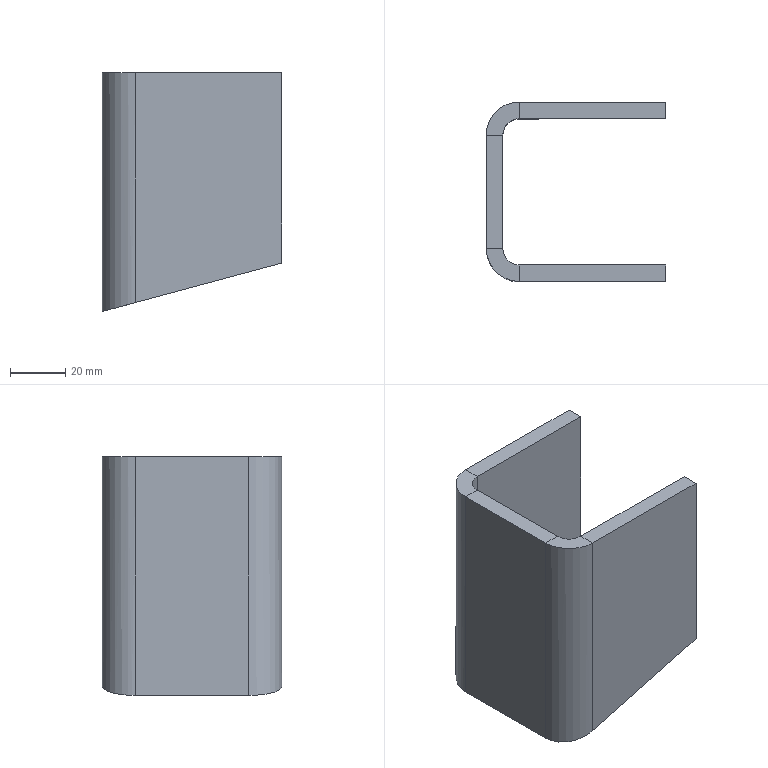Part | STEP file | 09-Bent plate | 1 solid | 18 faces | box 65 x 65 x 86.5 mm | volume 83900 mm3 | plane 14 | cylinder 4 | commonest cylinder face diameters 12 x2 24 x2
STEP:
#1=CARTESIAN_POINT('',(0.,0.,0.));
#2=DIRECTION('',(0.,0.,1.));
#3=DIRECTION('',(1.,0.,0.));
#4=AXIS2_PLACEMENT_3D('',#1,#2,#3);
#5=CARTESIAN_POINT('',(-53.,0.,86.5));
#6=VERTEX_POINT('',#5);
#7=CARTESIAN_POINT('',(-53.,-6.,86.5));
#8=VERTEX_POINT('',#7);
#9=CARTESIAN_POINT('',(-53.,0.,86.5));
#10=DIRECTION('',(0.,-1.,0.));
#11=VECTOR('',#10,1.);
#12=LINE('',#9,#11);
#13=CARTESIAN_POINT('',(-53.,0.,86.5));
#14=DIRECTION('',(0.,0.,1.));
#15=DIRECTION('',(1.,0.,0.));
#16=AXIS2_PLACEMENT_3D('',#13,#14,#15);
#17=PLANE('',#16);
#18=CARTESIAN_POINT('',(0.,0.));
#19=DIRECTION('',(0.,-1.));
#20=VECTOR('',#19,1.);
#21=LINE('',#18,#20);
#22=(GEOMETRIC_REPRESENTATION_CONTEXT(2)PARAMETRIC_REPRESENTATION_CONTEXT()REPRESENTATION_CONTEXT('',''));
#23=DEFINITIONAL_REPRESENTATION('',(#21),#22);
#24=PCURVE('',#17,#23);
#25=CARTESIAN_POINT('',(-59.,-12.,86.5));
#26=DIRECTION('',(0.,0.,1.));
#27=DIRECTION('',(1.,0.,0.));
#28=AXIS2_PLACEMENT_3D('',#25,#26,#27);
#29=PLANE('',#28);
#30=CARTESIAN_POINT('',(6.,12.));
#31=DIRECTION('',(0.,-1.));
#32=VECTOR('',#31,1.);
#33=LINE('',#30,#32);
#34=(GEOMETRIC_REPRESENTATION_CONTEXT(2)PARAMETRIC_REPRESENTATION_CONTEXT()REPRESENTATION_CONTEXT('',''));
#35=DEFINITIONAL_REPRESENTATION('',(#33),#34);
#36=PCURVE('',#29,#35);
#37=SURFACE_CURVE('',#12,(#24,#36),.PCURVE_S1.);
#38=EDGE_CURVE('',#6,#8,#37,.T.);
#39=ORIENTED_EDGE('',*,*,#38,.F.);
#40=CARTESIAN_POINT('',(-65.,-12.,86.5));
#41=VERTEX_POINT('',#40);
#42=CARTESIAN_POINT('',(-53.,-12.,86.5));
#43=DIRECTION('',(0.,0.,1.));
#44=DIRECTION('',(-1.,0.,0.));
#45=AXIS2_PLACEMENT_3D('',#42,#43,#44);
#46=CIRCLE('',#45,12.);
#47=CARTESIAN_POINT('',(0.,-12.));
#48=DIRECTION('',(-1.,0.));
#49=AXIS2_PLACEMENT_2D('',#47,#48);
#50=CIRCLE('',#49,12.);
#51=(GEOMETRIC_REPRESENTATION_CONTEXT(2)PARAMETRIC_REPRESENTATION_CONTEXT()REPRESENTATION_CONTEXT('',''));
#52=DEFINITIONAL_REPRESENTATION('',(#50),#51);
#53=PCURVE('',#17,#52);
#54=CARTESIAN_POINT('',(-53.,-12.,86.5));
#55=DIRECTION('',(0.,0.,-1.));
#56=DIRECTION('',(-1.,0.,0.));
#57=AXIS2_PLACEMENT_3D('',#54,#55,#56);
#58=CYLINDRICAL_SURFACE('',#57,12.);
#59=CARTESIAN_POINT('',(6.283,0.));
#60=DIRECTION('',(-1.,0.));
#61=VECTOR('',#60,1.);
#62=LINE('',#59,#61);
#63=(GEOMETRIC_REPRESENTATION_CONTEXT(2)PARAMETRIC_REPRESENTATION_CONTEXT()REPRESENTATION_CONTEXT('',''));
#64=DEFINITIONAL_REPRESENTATION('',(#62),#63);
#65=PCURVE('',#58,#64);
#66=SURFACE_CURVE('',#46,(#53,#65),.PCURVE_S1.);
#67=EDGE_CURVE('',#6,#41,#66,.T.);
#68=ORIENTED_EDGE('',*,*,#67,.T.);
#69=CARTESIAN_POINT('',(-59.,-12.,86.5));
#70=VERTEX_POINT('',#69);
#71=CARTESIAN_POINT('',(-59.,-12.,86.5));
#72=DIRECTION('',(-1.,0.,0.));
#73=VECTOR('',#72,1.);
#74=LINE('',#71,#73);
#75=CARTESIAN_POINT('',(-6.,-12.));
#76=DIRECTION('',(-1.,0.));
#77=VECTOR('',#76,1.);
#78=LINE('',#75,#77);
#79=(GEOMETRIC_REPRESENTATION_CONTEXT(2)PARAMETRIC_REPRESENTATION_CONTEXT()REPRESENTATION_CONTEXT('',''));
#80=DEFINITIONAL_REPRESENTATION('',(#78),#79);
#81=PCURVE('',#17,#80);
#82=CARTESIAN_POINT('',(-53.,-59.,86.5));
#83=DIRECTION('',(0.,0.,1.));
#84=DIRECTION('',(1.,0.,0.));
#85=AXIS2_PLACEMENT_3D('',#82,#83,#84);
#86=PLANE('',#85);
#87=CARTESIAN_POINT('',(-6.,47.));
#88=DIRECTION('',(-1.,0.));
#89=VECTOR('',#88,1.);
#90=LINE('',#87,#89);
#91=(GEOMETRIC_REPRESENTATION_CONTEXT(2)PARAMETRIC_REPRESENTATION_CONTEXT()REPRESENTATION_CONTEXT('',''));
#92=DEFINITIONAL_REPRESENTATION('',(#90),#91);
#93=PCURVE('',#86,#92);
#94=SURFACE_CURVE('',#74,(#81,#93),.PCURVE_S1.);
#95=EDGE_CURVE('',#70,#41,#94,.T.);
#96=ORIENTED_EDGE('',*,*,#95,.F.);
#97=CARTESIAN_POINT('',(-53.,-12.,86.5));
#98=DIRECTION('',(0.,0.,1.));
#99=DIRECTION('',(1.,0.,0.));
#100=AXIS2_PLACEMENT_3D('',#97,#98,#99);
#101=CIRCLE('',#100,6.);
#102=CARTESIAN_POINT('',(0.,-12.));
#103=DIRECTION('',(1.,0.));
#104=AXIS2_PLACEMENT_2D('',#102,#103);
#105=CIRCLE('',#104,6.);
#106=(GEOMETRIC_REPRESENTATION_CONTEXT(2)PARAMETRIC_REPRESENTATION_CONTEXT()REPRESENTATION_CONTEXT('',''));
#107=DEFINITIONAL_REPRESENTATION('',(#105),#106);
#108=PCURVE('',#17,#107);
#109=CARTESIAN_POINT('',(-53.,-12.,86.5));
#110=DIRECTION('',(0.,0.,-1.));
#111=DIRECTION('',(-1.,0.,0.));
#112=AXIS2_PLACEMENT_3D('',#109,#110,#111);
#113=CYLINDRICAL_SURFACE('',#112,6.);
#114=CARTESIAN_POINT('',(3.142,0.));
#115=DIRECTION('',(-1.,0.));
#116=VECTOR('',#115,1.);
#117=LINE('',#114,#116);
#118=(GEOMETRIC_REPRESENTATION_CONTEXT(2)PARAMETRIC_REPRESENTATION_CONTEXT()REPRESENTATION_CONTEXT('',''));
#119=DEFINITIONAL_REPRESENTATION('',(#117),#118);
#120=PCURVE('',#113,#119);
#121=SURFACE_CURVE('',#101,(#108,#120),.PCURVE_S1.);
#122=EDGE_CURVE('',#8,#70,#121,.T.);
#123=ORIENTED_EDGE('',*,*,#122,.F.);
#124=EDGE_LOOP('',(#39,#68,#96,#123));
#125=FACE_BOUND('',#124,.T.);
#126=ADVANCED_FACE('',(#125),#17,.T.);
#127=CARTESIAN_POINT('',(0.,0.,86.5));
#128=VERTEX_POINT('',#127);
#129=CARTESIAN_POINT('',(0.,0.,86.5));
#130=DIRECTION('',(-1.,0.,0.));
#131=VECTOR('',#130,1.);
#132=LINE('',#129,#131);
#133=CARTESIAN_POINT('',(59.,12.));
#134=DIRECTION('',(-1.,0.));
#135=VECTOR('',#134,1.);
#136=LINE('',#133,#135);
#137=(GEOMETRIC_REPRESENTATION_CONTEXT(2)PARAMETRIC_REPRESENTATION_CONTEXT()REPRESENTATION_CONTEXT('',''));
#138=DEFINITIONAL_REPRESENTATION('',(#136),#137);
#139=PCURVE('',#29,#138);
#140=CARTESIAN_POINT('',(0.,0.,86.5));
#141=DIRECTION('',(0.,-1.,0.));
#142=DIRECTION('',(1.,0.,0.));
#143=AXIS2_PLACEMENT_3D('',#140,#141,#142);
#144=PLANE('',#143);
#145=CARTESIAN_POINT('',(0.,0.));
#146=DIRECTION('',(-1.,0.));
#147=VECTOR('',#146,1.);
#148=LINE('',#145,#147);
#149=(GEOMETRIC_REPRESENTATION_CONTEXT(2)PARAMETRIC_REPRESENTATION_CONTEXT()REPRESENTATION_CONTEXT('',''));
#150=DEFINITIONAL_REPRESENTATION('',(#148),#149);
#151=PCURVE('',#144,#150);
#152=SURFACE_CURVE('',#132,(#139,#151),.PCURVE_S1.);
#153=EDGE_CURVE('',#128,#6,#152,.T.);
#154=ORIENTED_EDGE('',*,*,#153,.T.);
#155=ORIENTED_EDGE('',*,*,#38,.T.);
#156=CARTESIAN_POINT('',(0.,-6.,86.5));
#157=VERTEX_POINT('',#156);
#158=CARTESIAN_POINT('',(0.,-6.,86.5));
#159=DIRECTION('',(-1.,0.,0.));
#160=VECTOR('',#159,1.);
#161=LINE('',#158,#160);
#162=CARTESIAN_POINT('',(59.,6.));
#163=DIRECTION('',(-1.,0.));
#164=VECTOR('',#163,1.);
#165=LINE('',#162,#164);
#166=(GEOMETRIC_REPRESENTATION_CONTEXT(2)PARAMETRIC_REPRESENTATION_CONTEXT()REPRESENTATION_CONTEXT('',''));
#167=DEFINITIONAL_REPRESENTATION('',(#165),#166);
#168=PCURVE('',#29,#167);
#169=CARTESIAN_POINT('',(0.,-6.,86.5));
#170=DIRECTION('',(0.,-1.,0.));
#171=DIRECTION('',(1.,0.,0.));
#172=AXIS2_PLACEMENT_3D('',#169,#170,#171);
#173=PLANE('',#172);
#174=CARTESIAN_POINT('',(0.,0.));
#175=DIRECTION('',(-1.,0.));
#176=VECTOR('',#175,1.);
#177=LINE('',#174,#176);
#178=(GEOMETRIC_REPRESENTATION_CONTEXT(2)PARAMETRIC_REPRESENTATION_CONTEXT()REPRESENTATION_CONTEXT('',''));
#179=DEFINITIONAL_REPRESENTATION('',(#177),#178);
#180=PCURVE('',#173,#179);
#181=SURFACE_CURVE('',#161,(#168,#180),.PCURVE_S1.);
#182=EDGE_CURVE('',#157,#8,#181,.T.);
#183=ORIENTED_EDGE('',*,*,#182,.F.);
#184=CARTESIAN_POINT('',(0.,0.,86.5));
#185=DIRECTION('',(0.,-1.,0.));
#186=VECTOR('',#185,1.);
#187=LINE('',#184,#186);
#188=CARTESIAN_POINT('',(59.,12.));
#189=DIRECTION('',(0.,-1.));
#190=VECTOR('',#189,1.);
#191=LINE('',#188,#190);
#192=(GEOMETRIC_REPRESENTATION_CONTEXT(2)PARAMETRIC_REPRESENTATION_CONTEXT()REPRESENTATION_CONTEXT('',''));
#193=DEFINITIONAL_REPRESENTATION('',(#191),#192);
#194=PCURVE('',#29,#193);
#195=CARTESIAN_POINT('',(0.,0.,86.5));
#196=DIRECTION('',(1.,0.,0.));
#197=DIRECTION('',(0.,1.,0.));
#198=AXIS2_PLACEMENT_3D('',#195,#196,#197);
#199=PLANE('',#198);
#200=CARTESIAN_POINT('',(0.,0.));
#201=DIRECTION('',(-1.,0.));
#202=VECTOR('',#201,1.);
#203=LINE('',#200,#202);
#204=(GEOMETRIC_REPRESENTATION_CONTEXT(2)PARAMETRIC_REPRESENTATION_CONTEXT()REPRESENTATION_CONTEXT('',''));
#205=DEFINITIONAL_REPRESENTATION('',(#203),#204);
#206=PCURVE('',#199,#205);
#207=SURFACE_CURVE('',#187,(#194,#206),.PCURVE_S1.);
#208=EDGE_CURVE('',#128,#157,#207,.T.);
#209=ORIENTED_EDGE('',*,*,#208,.F.);
#210=EDGE_LOOP('',(#154,#155,#183,#209));
#211=FACE_BOUND('',#210,.T.);
#212=ADVANCED_FACE('',(#211),#29,.T.);
#213=CARTESIAN_POINT('',(-65.,-53.,86.5));
#214=VERTEX_POINT('',#213);
#215=CARTESIAN_POINT('',(-59.,-53.,86.5));
#216=VERTEX_POINT('',#215);
#217=CARTESIAN_POINT('',(-65.,-53.,86.5));
#218=DIRECTION('',(1.,0.,0.));
#219=VECTOR('',#218,1.);
#220=LINE('',#217,#219);
#221=CARTESIAN_POINT('',(-65.,-53.,86.5));
#222=DIRECTION('',(0.,0.,1.));
#223=DIRECTION('',(1.,0.,0.));
#224=AXIS2_PLACEMENT_3D('',#221,#222,#223);
#225=PLANE('',#224);
#226=CARTESIAN_POINT('',(0.,0.));
#227=DIRECTION('',(1.,0.));
#228=VECTOR('',#227,1.);
#229=LINE('',#226,#228);
#230=(GEOMETRIC_REPRESENTATION_CONTEXT(2)PARAMETRIC_REPRESENTATION_CONTEXT()REPRESENTATION_CONTEXT('',''));
#231=DEFINITIONAL_REPRESENTATION('',(#229),#230);
#232=PCURVE('',#225,#231);
#233=CARTESIAN_POINT('',(-12.,6.));
#234=DIRECTION('',(1.,0.));
#235=VECTOR('',#234,1.);
#236=LINE('',#233,#235);
#237=(GEOMETRIC_REPRESENTATION_CONTEXT(2)PARAMETRIC_REPRESENTATION_CONTEXT()REPRESENTATION_CONTEXT('',''));
#238=DEFINITIONAL_REPRESENTATION('',(#236),#237);
#239=PCURVE('',#86,#238);
#240=SURFACE_CURVE('',#220,(#232,#239),.PCURVE_S1.);
#241=EDGE_CURVE('',#214,#216,#240,.T.);
#242=ORIENTED_EDGE('',*,*,#241,.F.);
#243=CARTESIAN_POINT('',(-53.,-65.,86.5));
#244=VERTEX_POINT('',#243);
#245=CARTESIAN_POINT('',(-53.,-53.,86.5));
#246=DIRECTION('',(0.,0.,1.));
#247=DIRECTION('',(-1.,0.,0.));
#248=AXIS2_PLACEMENT_3D('',#245,#246,#247);
#249=CIRCLE('',#248,12.);
#250=CARTESIAN_POINT('',(12.,0.));
#251=DIRECTION('',(-1.,0.));
#252=AXIS2_PLACEMENT_2D('',#250,#251);
#253=CIRCLE('',#252,12.);
#254=(GEOMETRIC_REPRESENTATION_CONTEXT(2)PARAMETRIC_REPRESENTATION_CONTEXT()REPRESENTATION_CONTEXT('',''));
#255=DEFINITIONAL_REPRESENTATION('',(#253),#254);
#256=PCURVE('',#225,#255);
#257=CARTESIAN_POINT('',(-53.,-53.,86.5));
#258=DIRECTION('',(0.,0.,-1.));
#259=DIRECTION('',(-1.,0.,0.));
#260=AXIS2_PLACEMENT_3D('',#257,#258,#259);
#261=CYLINDRICAL_SURFACE('',#260,12.);
#262=CARTESIAN_POINT('',(6.283,0.));
#263=DIRECTION('',(-1.,0.));
#264=VECTOR('',#263,1.);
#265=LINE('',#262,#264);
#266=(GEOMETRIC_REPRESENTATION_CONTEXT(2)PARAMETRIC_REPRESENTATION_CONTEXT()REPRESENTATION_CONTEXT('',''));
#267=DEFINITIONAL_REPRESENTATION('',(#265),#266);
#268=PCURVE('',#261,#267);
#269=SURFACE_CURVE('',#249,(#256,#268),.PCURVE_S1.);
#270=EDGE_CURVE('',#214,#244,#269,.T.);
#271=ORIENTED_EDGE('',*,*,#270,.T.);
#272=CARTESIAN_POINT('',(-53.,-59.,86.5));
#273=VERTEX_POINT('',#272);
#274=CARTESIAN_POINT('',(-53.,-59.,86.5));
#275=DIRECTION('',(0.,-1.,0.));
#276=VECTOR('',#275,1.);
#277=LINE('',#274,#276);
#278=CARTESIAN_POINT('',(12.,-6.));
#279=DIRECTION('',(0.,-1.));
#280=VECTOR('',#279,1.);
#281=LINE('',#278,#280);
#282=(GEOMETRIC_REPRESENTATION_CONTEXT(2)PARAMETRIC_REPRESENTATION_CONTEXT()REPRESENTATION_CONTEXT('',''));
#283=DEFINITIONAL_REPRESENTATION('',(#281),#282);
#284=PCURVE('',#225,#283);
#285=CARTESIAN_POINT('',(-53.,-53.,86.5));
#286=DIRECTION('',(0.,0.,1.));
#287=DIRECTION('',(1.,0.,0.));
#288=AXIS2_PLACEMENT_3D('',#285,#286,#287);
#289=PLANE('',#288);
#290=CARTESIAN_POINT('',(0.,-6.));
#291=DIRECTION('',(0.,-1.));
#292=VECTOR('',#291,1.);
#293=LINE('',#290,#292);
#294=(GEOMETRIC_REPRESENTATION_CONTEXT(2)PARAMETRIC_REPRESENTATION_CONTEXT()REPRESENTATION_CONTEXT('',''));
#295=DEFINITIONAL_REPRESENTATION('',(#293),#294);
#296=PCURVE('',#289,#295);
#297=SURFACE_CURVE('',#277,(#284,#296),.PCURVE_S1.);
#298=EDGE_CURVE('',#273,#244,#297,.T.);
#299=ORIENTED_EDGE('',*,*,#298,.F.);
#300=CARTESIAN_POINT('',(-53.,-53.,86.5));
#301=DIRECTION('',(0.,0.,1.));
#302=DIRECTION('',(1.,0.,0.));
#303=AXIS2_PLACEMENT_3D('',#300,#301,#302);
#304=CIRCLE('',#303,6.);
#305=CARTESIAN_POINT('',(12.,0.));
#306=DIRECTION('',(1.,0.));
#307=AXIS2_PLACEMENT_2D('',#305,#306);
#308=CIRCLE('',#307,6.);
#309=(GEOMETRIC_REPRESENTATION_CONTEXT(2)PARAMETRIC_REPRESENTATION_CONTEXT()REPRESENTATION_CONTEXT('',''));
#310=DEFINITIONAL_REPRESENTATION('',(#308),#309);
#311=PCURVE('',#225,#310);
#312=CARTESIAN_POINT('',(-53.,-53.,86.5));
#313=DIRECTION('',(0.,0.,-1.));
#314=DIRECTION('',(-1.,0.,0.));
#315=AXIS2_PLACEMENT_3D('',#312,#313,#314);
#316=CYLINDRICAL_SURFACE('',#315,6.);
#317=CARTESIAN_POINT('',(9.425,0.));
#318=DIRECTION('',(-1.,0.));
#319=VECTOR('',#318,1.);
#320=LINE('',#317,#319);
#321=(GEOMETRIC_REPRESENTATION_CONTEXT(2)PARAMETRIC_REPRESENTATION_CONTEXT()REPRESENTATION_CONTEXT('',''));
#322=DEFINITIONAL_REPRESENTATION('',(#320),#321);
#323=PCURVE('',#316,#322);
#324=SURFACE_CURVE('',#304,(#311,#323),.PCURVE_S1.);
#325=EDGE_CURVE('',#216,#273,#324,.T.);
#326=ORIENTED_EDGE('',*,*,#325,.F.);
#327=EDGE_LOOP('',(#242,#271,#299,#326));
#328=FACE_BOUND('',#327,.T.);
#329=ADVANCED_FACE('',(#328),#225,.T.);
#330=CARTESIAN_POINT('',(-65.,0.,86.5));
#331=DIRECTION('',(0.,-1.,0.));
#332=VECTOR('',#331,1.);
#333=LINE('',#330,#332);
#334=CARTESIAN_POINT('',(-12.,59.));
#335=DIRECTION('',(0.,-1.));
#336=VECTOR('',#335,1.);
#337=LINE('',#334,#336);
#338=(GEOMETRIC_REPRESENTATION_CONTEXT(2)PARAMETRIC_REPRESENTATION_CONTEXT()REPRESENTATION_CONTEXT('',''));
#339=DEFINITIONAL_REPRESENTATION('',(#337),#338);
#340=PCURVE('',#86,#339);
#341=CARTESIAN_POINT('',(-65.,0.,86.5));
#342=DIRECTION('',(1.,0.,0.));
#343=DIRECTION('',(0.,1.,0.));
#344=AXIS2_PLACEMENT_3D('',#341,#342,#343);
#345=PLANE('',#344);
#346=CARTESIAN_POINT('',(0.,0.));
#347=DIRECTION('',(-1.,0.));
#348=VECTOR('',#347,1.);
#349=LINE('',#346,#348);
#350=(GEOMETRIC_REPRESENTATION_CONTEXT(2)PARAMETRIC_REPRESENTATION_CONTEXT()REPRESENTATION_CONTEXT('',''));
#351=DEFINITIONAL_REPRESENTATION('',(#349),#350);
#352=PCURVE('',#345,#351);
#353=SURFACE_CURVE('',#333,(#340,#352),.PCURVE_S1.);
#354=EDGE_CURVE('',#41,#214,#353,.T.);
#355=ORIENTED_EDGE('',*,*,#354,.T.);
#356=ORIENTED_EDGE('',*,*,#241,.T.);
#357=CARTESIAN_POINT('',(-59.,0.,86.5));
#358=DIRECTION('',(0.,-1.,0.));
#359=VECTOR('',#358,1.);
#360=LINE('',#357,#359);
#361=CARTESIAN_POINT('',(-6.,59.));
#362=DIRECTION('',(0.,-1.));
#363=VECTOR('',#362,1.);
#364=LINE('',#361,#363);
#365=(GEOMETRIC_REPRESENTATION_CONTEXT(2)PARAMETRIC_REPRESENTATION_CONTEXT()REPRESENTATION_CONTEXT('',''));
#366=DEFINITIONAL_REPRESENTATION('',(#364),#365);
#367=PCURVE('',#86,#366);
#368=CARTESIAN_POINT('',(-59.,0.,86.5));
#369=DIRECTION('',(1.,0.,0.));
#370=DIRECTION('',(0.,1.,0.));
#371=AXIS2_PLACEMENT_3D('',#368,#369,#370);
#372=PLANE('',#371);
#373=CARTESIAN_POINT('',(0.,0.));
#374=DIRECTION('',(-1.,0.));
#375=VECTOR('',#374,1.);
#376=LINE('',#373,#375);
#377=(GEOMETRIC_REPRESENTATION_CONTEXT(2)PARAMETRIC_REPRESENTATION_CONTEXT()REPRESENTATION_CONTEXT('',''));
#378=DEFINITIONAL_REPRESENTATION('',(#376),#377);
#379=PCURVE('',#372,#378);
#380=SURFACE_CURVE('',#360,(#367,#379),.PCURVE_S1.);
#381=EDGE_CURVE('',#70,#216,#380,.T.);
#382=ORIENTED_EDGE('',*,*,#381,.F.);
#383=ORIENTED_EDGE('',*,*,#95,.T.);
#384=EDGE_LOOP('',(#355,#356,#382,#383));
#385=FACE_BOUND('',#384,.T.);
#386=ADVANCED_FACE('',(#385),#86,.T.);
#387=CARTESIAN_POINT('',(-53.,-65.,3.231));
#388=VERTEX_POINT('',#387);
#389=CARTESIAN_POINT('',(-53.,-65.,86.5));
#390=DIRECTION('',(0.,0.,-1.));
#391=VECTOR('',#390,1.);
#392=LINE('',#389,#391);
#393=CARTESIAN_POINT('',(-65.,-65.,86.5));
#394=DIRECTION('',(0.,1.,0.));
#395=DIRECTION('',(0.,0.,1.));
#396=AXIS2_PLACEMENT_3D('',#393,#394,#395);
#397=PLANE('',#396);
#398=CARTESIAN_POINT('',(0.,12.));
#399=DIRECTION('',(-1.,0.));
#400=VECTOR('',#399,1.);
#401=LINE('',#398,#400);
#402=(GEOMETRIC_REPRESENTATION_CONTEXT(2)PARAMETRIC_REPRESENTATION_CONTEXT()REPRESENTATION_CONTEXT('',''));
#403=DEFINITIONAL_REPRESENTATION('',(#401),#402);
#404=PCURVE('',#397,#403);
#405=CARTESIAN_POINT('',(4.712,0.));
#406=DIRECTION('',(0.,1.));
#407=VECTOR('',#406,1.);
#408=LINE('',#405,#407);
#409=(GEOMETRIC_REPRESENTATION_CONTEXT(2)PARAMETRIC_REPRESENTATION_CONTEXT()REPRESENTATION_CONTEXT('',''));
#410=DEFINITIONAL_REPRESENTATION('',(#408),#409);
#411=PCURVE('',#261,#410);
#412=SURFACE_CURVE('',#392,(#404,#411),.PCURVE_S1.);
#413=EDGE_CURVE('',#244,#388,#412,.T.);
#414=ORIENTED_EDGE('',*,*,#413,.T.);
#415=CARTESIAN_POINT('',(0.,-65.,17.5));
#416=VERTEX_POINT('',#415);
#417=CARTESIAN_POINT('',(-4.393,-65.,16.317));
#418=DIRECTION('',(0.9656,0.,0.26));
#419=VECTOR('',#418,1.);
#420=LINE('',#417,#419);
#421=CARTESIAN_POINT('',(-70.183,60.607));
#422=DIRECTION('',(0.26,0.9656));
#423=VECTOR('',#422,1.);
#424=LINE('',#421,#423);
#425=(GEOMETRIC_REPRESENTATION_CONTEXT(2)PARAMETRIC_REPRESENTATION_CONTEXT()REPRESENTATION_CONTEXT('',''));
#426=DEFINITIONAL_REPRESENTATION('',(#424),#425);
#427=PCURVE('',#397,#426);
#428=CARTESIAN_POINT('',(-4.393,-65.,16.317));
#429=DIRECTION('',(-0.26,0.,0.9656));
#430=DIRECTION('',(0.9656,0.,0.26));
#431=AXIS2_PLACEMENT_3D('',#428,#429,#430);
#432=PLANE('',#431);
#433=CARTESIAN_POINT('',(0.,0.));
#434=DIRECTION('',(1.,0.));
#435=VECTOR('',#434,1.);
#436=LINE('',#433,#435);
#437=(GEOMETRIC_REPRESENTATION_CONTEXT(2)PARAMETRIC_REPRESENTATION_CONTEXT()REPRESENTATION_CONTEXT('',''));
#438=DEFINITIONAL_REPRESENTATION('',(#436),#437);
#439=PCURVE('',#432,#438);
#440=SURFACE_CURVE('',#420,(#427,#439),.PCURVE_S1.);
#441=EDGE_CURVE('',#388,#416,#440,.T.);
#442=ORIENTED_EDGE('',*,*,#441,.T.);
#443=CARTESIAN_POINT('',(0.,-65.,86.5));
#444=VERTEX_POINT('',#443);
#445=CARTESIAN_POINT('',(0.,-65.,86.5));
#446=DIRECTION('',(0.,0.,-1.));
#447=VECTOR('',#446,1.);
#448=LINE('',#445,#447);
#449=CARTESIAN_POINT('',(0.,65.));
#450=DIRECTION('',(-1.,0.));
#451=VECTOR('',#450,1.);
#452=LINE('',#449,#451);
#453=(GEOMETRIC_REPRESENTATION_CONTEXT(2)PARAMETRIC_REPRESENTATION_CONTEXT()REPRESENTATION_CONTEXT('',''));
#454=DEFINITIONAL_REPRESENTATION('',(#452),#453);
#455=PCURVE('',#397,#454);
#456=CARTESIAN_POINT('',(0.,-59.,86.5));
#457=DIRECTION('',(1.,0.,0.));
#458=DIRECTION('',(0.,0.,-1.));
#459=AXIS2_PLACEMENT_3D('',#456,#457,#458);
#460=PLANE('',#459);
#461=CARTESIAN_POINT('',(0.,-6.));
#462=DIRECTION('',(1.,0.));
#463=VECTOR('',#462,1.);
#464=LINE('',#461,#463);
#465=(GEOMETRIC_REPRESENTATION_CONTEXT(2)PARAMETRIC_REPRESENTATION_CONTEXT()REPRESENTATION_CONTEXT('',''));
#466=DEFINITIONAL_REPRESENTATION('',(#464),#465);
#467=PCURVE('',#460,#466);
#468=SURFACE_CURVE('',#448,(#455,#467),.PCURVE_S1.);
#469=EDGE_CURVE('',#444,#416,#468,.T.);
#470=ORIENTED_EDGE('',*,*,#469,.F.);
#471=CARTESIAN_POINT('',(-65.,-65.,86.5));
#472=DIRECTION('',(1.,0.,0.));
#473=VECTOR('',#472,1.);
#474=LINE('',#471,#473);
#475=CARTESIAN_POINT('',(0.,0.));
#476=DIRECTION('',(0.,1.));
#477=VECTOR('',#476,1.);
#478=LINE('',#475,#477);
#479=(GEOMETRIC_REPRESENTATION_CONTEXT(2)PARAMETRIC_REPRESENTATION_CONTEXT()REPRESENTATION_CONTEXT('',''));
#480=DEFINITIONAL_REPRESENTATION('',(#478),#479);
#481=PCURVE('',#397,#480);
#482=CARTESIAN_POINT('',(-12.,-12.));
#483=DIRECTION('',(1.,0.));
#484=VECTOR('',#483,1.);
#485=LINE('',#482,#484);
#486=(GEOMETRIC_REPRESENTATION_CONTEXT(2)PARAMETRIC_REPRESENTATION_CONTEXT()REPRESENTATION_CONTEXT('',''));
#487=DEFINITIONAL_REPRESENTATION('',(#485),#486);
#488=PCURVE('',#289,#487);
#489=SURFACE_CURVE('',#474,(#481,#488),.PCURVE_S1.);
#490=EDGE_CURVE('',#244,#444,#489,.T.);
#491=ORIENTED_EDGE('',*,*,#490,.F.);
#492=EDGE_LOOP('',(#414,#442,#470,#491));
#493=FACE_BOUND('',#492,.T.);
#494=ADVANCED_FACE('',(#493),#397,.F.);
#495=CARTESIAN_POINT('',(0.,-59.,17.5));
#496=VERTEX_POINT('',#495);
#497=CARTESIAN_POINT('',(0.,-65.,17.5));
#498=DIRECTION('',(0.,1.,0.));
#499=VECTOR('',#498,1.);
#500=LINE('',#497,#499);
#501=CARTESIAN_POINT('',(69.,-6.));
#502=DIRECTION('',(0.,1.));
#503=VECTOR('',#502,1.);
#504=LINE('',#501,#503);
#505=(GEOMETRIC_REPRESENTATION_CONTEXT(2)PARAMETRIC_REPRESENTATION_CONTEXT()REPRESENTATION_CONTEXT('',''));
#506=DEFINITIONAL_REPRESENTATION('',(#504),#505);
#507=PCURVE('',#460,#506);
#508=CARTESIAN_POINT('',(4.55,0.));
#509=DIRECTION('',(0.,1.));
#510=VECTOR('',#509,1.);
#511=LINE('',#508,#510);
#512=(GEOMETRIC_REPRESENTATION_CONTEXT(2)PARAMETRIC_REPRESENTATION_CONTEXT()REPRESENTATION_CONTEXT('',''));
#513=DEFINITIONAL_REPRESENTATION('',(#511),#512);
#514=PCURVE('',#432,#513);
#515=SURFACE_CURVE('',#500,(#507,#514),.PCURVE_S1.);
#516=EDGE_CURVE('',#416,#496,#515,.T.);
#517=ORIENTED_EDGE('',*,*,#516,.T.);
#518=CARTESIAN_POINT('',(0.,-59.,86.5));
#519=VERTEX_POINT('',#518);
#520=CARTESIAN_POINT('',(0.,-59.,86.5));
#521=DIRECTION('',(0.,0.,-1.));
#522=VECTOR('',#521,1.);
#523=LINE('',#520,#522);
#524=CARTESIAN_POINT('',(0.,0.));
#525=DIRECTION('',(1.,0.));
#526=VECTOR('',#525,1.);
#527=LINE('',#524,#526);
#528=(GEOMETRIC_REPRESENTATION_CONTEXT(2)PARAMETRIC_REPRESENTATION_CONTEXT()REPRESENTATION_CONTEXT('',''));
#529=DEFINITIONAL_REPRESENTATION('',(#527),#528);
#530=PCURVE('',#460,#529);
#531=CARTESIAN_POINT('',(-65.,-59.,86.5));
#532=DIRECTION('',(0.,1.,0.));
#533=DIRECTION('',(0.,0.,1.));
#534=AXIS2_PLACEMENT_3D('',#531,#532,#533);
#535=PLANE('',#534);
#536=CARTESIAN_POINT('',(0.,65.));
#537=DIRECTION('',(-1.,0.));
#538=VECTOR('',#537,1.);
#539=LINE('',#536,#538);
#540=(GEOMETRIC_REPRESENTATION_CONTEXT(2)PARAMETRIC_REPRESENTATION_CONTEXT()REPRESENTATION_CONTEXT('',''));
#541=DEFINITIONAL_REPRESENTATION('',(#539),#540);
#542=PCURVE('',#535,#541);
#543=SURFACE_CURVE('',#523,(#530,#542),.PCURVE_S1.);
#544=EDGE_CURVE('',#519,#496,#543,.T.);
#545=ORIENTED_EDGE('',*,*,#544,.F.);
#546=CARTESIAN_POINT('',(0.,-59.,86.5));
#547=DIRECTION('',(0.,-1.,0.));
#548=VECTOR('',#547,1.);
#549=LINE('',#546,#548);
#550=CARTESIAN_POINT('',(0.,0.));
#551=DIRECTION('',(0.,-1.));
#552=VECTOR('',#551,1.);
#553=LINE('',#550,#552);
#554=(GEOMETRIC_REPRESENTATION_CONTEXT(2)PARAMETRIC_REPRESENTATION_CONTEXT()REPRESENTATION_CONTEXT('',''));
#555=DEFINITIONAL_REPRESENTATION('',(#553),#554);
#556=PCURVE('',#460,#555);
#557=CARTESIAN_POINT('',(53.,-6.));
#558=DIRECTION('',(0.,-1.));
#559=VECTOR('',#558,1.);
#560=LINE('',#557,#559);
#561=(GEOMETRIC_REPRESENTATION_CONTEXT(2)PARAMETRIC_REPRESENTATION_CONTEXT()REPRESENTATION_CONTEXT('',''));
#562=DEFINITIONAL_REPRESENTATION('',(#560),#561);
#563=PCURVE('',#289,#562);
#564=SURFACE_CURVE('',#549,(#556,#563),.PCURVE_S1.);
#565=EDGE_CURVE('',#519,#444,#564,.T.);
#566=ORIENTED_EDGE('',*,*,#565,.T.);
#567=ORIENTED_EDGE('',*,*,#469,.T.);
#568=EDGE_LOOP('',(#517,#545,#566,#567));
#569=FACE_BOUND('',#568,.T.);
#570=ADVANCED_FACE('',(#569),#460,.T.);
#571=CARTESIAN_POINT('',(-53.,-59.,3.231));
#572=VERTEX_POINT('',#571);
#573=CARTESIAN_POINT('',(-43.286,-59.,5.846));
#574=DIRECTION('',(0.9656,0.,0.26));
#575=VECTOR('',#574,1.);
#576=LINE('',#573,#575);
#577=CARTESIAN_POINT('',(-80.654,21.714));
#578=DIRECTION('',(0.26,0.9656));
#579=VECTOR('',#578,1.);
#580=LINE('',#577,#579);
#581=(GEOMETRIC_REPRESENTATION_CONTEXT(2)PARAMETRIC_REPRESENTATION_CONTEXT()REPRESENTATION_CONTEXT('',''));
#582=DEFINITIONAL_REPRESENTATION('',(#580),#581);
#583=PCURVE('',#535,#582);
#584=CARTESIAN_POINT('',(-40.277,6.));
#585=DIRECTION('',(1.,0.));
#586=VECTOR('',#585,1.);
#587=LINE('',#584,#586);
#588=(GEOMETRIC_REPRESENTATION_CONTEXT(2)PARAMETRIC_REPRESENTATION_CONTEXT()REPRESENTATION_CONTEXT('',''));
#589=DEFINITIONAL_REPRESENTATION('',(#587),#588);
#590=PCURVE('',#432,#589);
#591=SURFACE_CURVE('',#576,(#583,#590),.PCURVE_S1.);
#592=EDGE_CURVE('',#572,#496,#591,.T.);
#593=ORIENTED_EDGE('',*,*,#592,.F.);
#594=CARTESIAN_POINT('',(-53.,-59.,86.5));
#595=DIRECTION('',(0.,0.,-1.));
#596=VECTOR('',#595,1.);
#597=LINE('',#594,#596);
#598=CARTESIAN_POINT('',(0.,12.));
#599=DIRECTION('',(-1.,0.));
#600=VECTOR('',#599,1.);
#601=LINE('',#598,#600);
#602=(GEOMETRIC_REPRESENTATION_CONTEXT(2)PARAMETRIC_REPRESENTATION_CONTEXT()REPRESENTATION_CONTEXT('',''));
#603=DEFINITIONAL_REPRESENTATION('',(#601),#602);
#604=PCURVE('',#535,#603);
#605=CARTESIAN_POINT('',(4.712,0.));
#606=DIRECTION('',(0.,1.));
#607=VECTOR('',#606,1.);
#608=LINE('',#605,#607);
#609=(GEOMETRIC_REPRESENTATION_CONTEXT(2)PARAMETRIC_REPRESENTATION_CONTEXT()REPRESENTATION_CONTEXT('',''));
#610=DEFINITIONAL_REPRESENTATION('',(#608),#609);
#611=PCURVE('',#316,#610);
#612=SURFACE_CURVE('',#597,(#604,#611),.PCURVE_S1.);
#613=EDGE_CURVE('',#273,#572,#612,.T.);
#614=ORIENTED_EDGE('',*,*,#613,.F.);
#615=CARTESIAN_POINT('',(-65.,-59.,86.5));
#616=DIRECTION('',(1.,0.,0.));
#617=VECTOR('',#616,1.);
#618=LINE('',#615,#617);
#619=CARTESIAN_POINT('',(0.,0.));
#620=DIRECTION('',(0.,1.));
#621=VECTOR('',#620,1.);
#622=LINE('',#619,#621);
#623=(GEOMETRIC_REPRESENTATION_CONTEXT(2)PARAMETRIC_REPRESENTATION_CONTEXT()REPRESENTATION_CONTEXT('',''));
#624=DEFINITIONAL_REPRESENTATION('',(#622),#623);
#625=PCURVE('',#535,#624);
#626=CARTESIAN_POINT('',(-12.,-6.));
#627=DIRECTION('',(1.,0.));
#628=VECTOR('',#627,1.);
#629=LINE('',#626,#628);
#630=(GEOMETRIC_REPRESENTATION_CONTEXT(2)PARAMETRIC_REPRESENTATION_CONTEXT()REPRESENTATION_CONTEXT('',''));
#631=DEFINITIONAL_REPRESENTATION('',(#629),#630);
#632=PCURVE('',#289,#631);
#633=SURFACE_CURVE('',#618,(#625,#632),.PCURVE_S1.);
#634=EDGE_CURVE('',#273,#519,#633,.T.);
#635=ORIENTED_EDGE('',*,*,#634,.T.);
#636=ORIENTED_EDGE('',*,*,#544,.T.);
#637=EDGE_LOOP('',(#593,#614,#635,#636));
#638=FACE_BOUND('',#637,.T.);
#639=ADVANCED_FACE('',(#638),#535,.T.);
#640=ORIENTED_EDGE('',*,*,#613,.F.);
#641=ORIENTED_EDGE('',*,*,#325,.F.);
#642=CARTESIAN_POINT('',(-59.,-53.,1.615));
#643=VERTEX_POINT('',#642);
#644=CARTESIAN_POINT('',(-59.,-53.,86.5));
#645=DIRECTION('',(0.,0.,-1.));
#646=VECTOR('',#645,1.);
#647=LINE('',#644,#646);
#648=CARTESIAN_POINT('',(6.283,0.));
#649=DIRECTION('',(0.,1.));
#650=VECTOR('',#649,1.);
#651=LINE('',#648,#650);
#652=(GEOMETRIC_REPRESENTATION_CONTEXT(2)PARAMETRIC_REPRESENTATION_CONTEXT()REPRESENTATION_CONTEXT('',''));
#653=DEFINITIONAL_REPRESENTATION('',(#651),#652);
#654=PCURVE('',#316,#653);
#655=CARTESIAN_POINT('',(-53.,0.));
#656=DIRECTION('',(0.,-1.));
#657=VECTOR('',#656,1.);
#658=LINE('',#655,#657);
#659=(GEOMETRIC_REPRESENTATION_CONTEXT(2)PARAMETRIC_REPRESENTATION_CONTEXT()REPRESENTATION_CONTEXT('',''));
#660=DEFINITIONAL_REPRESENTATION('',(#658),#659);
#661=PCURVE('',#372,#660);
#662=SURFACE_CURVE('',#647,(#654,#661),.PCURVE_S1.);
#663=EDGE_CURVE('',#216,#643,#662,.T.);
#664=ORIENTED_EDGE('',*,*,#663,.T.);
#665=CARTESIAN_POINT('',(-59.,-53.,1.615));
#666=CARTESIAN_POINT('',(-59.,-56.515,1.615));
#667=CARTESIAN_POINT('',(-56.515,-59.,2.284));
#668=CARTESIAN_POINT('',(-53.,-59.,3.231));
#669=(BOUNDED_CURVE()B_SPLINE_CURVE(3,(#665,#666,#667,#668),.UNSPECIFIED.,.F.,.F.)B_SPLINE_CURVE_WITH_KNOTS((4,4),(0.,1.571),.PIECEWISE_BEZIER_KNOTS.)CURVE()GEOMETRIC_REPRESENTATION_ITEM()RATIONAL_B_SPLINE_CURVE((1.,0.8047,0.8047,1.))REPRESENTATION_ITEM(''));
#670=CARTESIAN_POINT('',(6.283,84.885));
#671=CARTESIAN_POINT('',(6.262,84.885));
#672=CARTESIAN_POINT('',(6.218,84.882));
#673=CARTESIAN_POINT('',(6.152,84.872));
#674=CARTESIAN_POINT('',(6.083,84.854));
#675=CARTESIAN_POINT('',(6.013,84.827));
#676=CARTESIAN_POINT('',(5.942,84.793));
#677=CARTESIAN_POINT('',(5.87,84.75));
#678=CARTESIAN_POINT('',(5.797,84.699));
#679=CARTESIAN_POINT('',(5.723,84.639));
#680=CARTESIAN_POINT('',(5.648,84.571));
#681=CARTESIAN_POINT('',(5.573,84.495));
#682=CARTESIAN_POINT('',(5.498,84.413));
#683=CARTESIAN_POINT('',(5.422,84.323));
#684=CARTESIAN_POINT('',(5.347,84.228));
#685=CARTESIAN_POINT('',(5.273,84.129));
#686=CARTESIAN_POINT('',(5.199,84.025));
#687=CARTESIAN_POINT('',(5.125,83.918));
#688=CARTESIAN_POINT('',(5.053,83.81));
#689=CARTESIAN_POINT('',(4.982,83.7));
#690=CARTESIAN_POINT('',(4.912,83.59));
#691=CARTESIAN_POINT('',(4.844,83.481));
#692=CARTESIAN_POINT('',(4.777,83.374));
#693=CARTESIAN_POINT('',(4.734,83.304));
#694=CARTESIAN_POINT('',(4.712,83.269));
#695=B_SPLINE_CURVE_WITH_KNOTS('',3,(#670,#671,#672,#673,#674,#675,#676,#677,#678,#679,#680,#681,#682,#683,#684,#685,#686,#687,#688,#689,#690,#691,#692,#693,#694),.UNSPECIFIED.,.F.,.F.,(4,1,1,1,1,1,1,1,1,1,1,1,1,1,1,1,1,1,1,1,1,1,4),(0.,0.0714,0.1428,0.2142,0.2856,0.357,0.4284,0.4998,0.5712,0.6426,0.714,0.7854,0.8568,0.9282,0.9996,1.071,1.142,1.214,1.285,1.357,1.428,1.499,1.571),.QUASI_UNIFORM_KNOTS.);
#696=(GEOMETRIC_REPRESENTATION_CONTEXT(2)PARAMETRIC_REPRESENTATION_CONTEXT()REPRESENTATION_CONTEXT('',''));
#697=DEFINITIONAL_REPRESENTATION('',(#695),#696);
#698=PCURVE('',#316,#697);
#699=CARTESIAN_POINT('',(-56.551,12.));
#700=CARTESIAN_POINT('',(-56.551,8.485));
#701=CARTESIAN_POINT('',(-53.978,6.));
#702=CARTESIAN_POINT('',(-50.338,6.));
#703=(BOUNDED_CURVE()B_SPLINE_CURVE(3,(#699,#700,#701,#702),.UNSPECIFIED.,.F.,.F.)B_SPLINE_CURVE_WITH_KNOTS((4,4),(0.,1.571),.PIECEWISE_BEZIER_KNOTS.)CURVE()GEOMETRIC_REPRESENTATION_ITEM()RATIONAL_B_SPLINE_CURVE((1.,0.8047,0.8047,1.))REPRESENTATION_ITEM(''));
#704=(GEOMETRIC_REPRESENTATION_CONTEXT(2)PARAMETRIC_REPRESENTATION_CONTEXT()REPRESENTATION_CONTEXT('',''));
#705=DEFINITIONAL_REPRESENTATION('',(#703),#704);
#706=PCURVE('',#432,#705);
#707=SURFACE_CURVE('',#669,(#698,#706),.PCURVE_S1.);
#708=EDGE_CURVE('',#643,#572,#707,.T.);
#709=ORIENTED_EDGE('',*,*,#708,.T.);
#710=EDGE_LOOP('',(#640,#641,#664,#709));
#711=FACE_BOUND('',#710,.F.);
#712=ADVANCED_FACE('',(#711),#316,.F.);
#713=CARTESIAN_POINT('',(-59.,-12.,1.615));
#714=VERTEX_POINT('',#713);
#715=CARTESIAN_POINT('',(-59.,0.,1.615));
#716=DIRECTION('',(0.,-1.,0.));
#717=VECTOR('',#716,1.);
#718=LINE('',#715,#717);
#719=CARTESIAN_POINT('',(0.,-84.885));
#720=DIRECTION('',(-1.,0.));
#721=VECTOR('',#720,1.);
#722=LINE('',#719,#721);
#723=(GEOMETRIC_REPRESENTATION_CONTEXT(2)PARAMETRIC_REPRESENTATION_CONTEXT()REPRESENTATION_CONTEXT('',''));
#724=DEFINITIONAL_REPRESENTATION('',(#722),#723);
#725=PCURVE('',#372,#724);
#726=CARTESIAN_POINT('',(-56.551,65.));
#727=DIRECTION('',(0.,-1.));
#728=VECTOR('',#727,1.);
#729=LINE('',#726,#728);
#730=(GEOMETRIC_REPRESENTATION_CONTEXT(2)PARAMETRIC_REPRESENTATION_CONTEXT()REPRESENTATION_CONTEXT('',''));
#731=DEFINITIONAL_REPRESENTATION('',(#729),#730);
#732=PCURVE('',#432,#731);
#733=SURFACE_CURVE('',#718,(#725,#732),.PCURVE_S1.);
#734=EDGE_CURVE('',#714,#643,#733,.T.);
#735=ORIENTED_EDGE('',*,*,#734,.F.);
#736=CARTESIAN_POINT('',(-59.,-12.,86.5));
#737=DIRECTION('',(0.,0.,-1.));
#738=VECTOR('',#737,1.);
#739=LINE('',#736,#738);
#740=CARTESIAN_POINT('',(-12.,0.));
#741=DIRECTION('',(0.,-1.));
#742=VECTOR('',#741,1.);
#743=LINE('',#740,#742);
#744=(GEOMETRIC_REPRESENTATION_CONTEXT(2)PARAMETRIC_REPRESENTATION_CONTEXT()REPRESENTATION_CONTEXT('',''));
#745=DEFINITIONAL_REPRESENTATION('',(#743),#744);
#746=PCURVE('',#372,#745);
#747=CARTESIAN_POINT('',(0.,0.));
#748=DIRECTION('',(0.,1.));
#749=VECTOR('',#748,1.);
#750=LINE('',#747,#749);
#751=(GEOMETRIC_REPRESENTATION_CONTEXT(2)PARAMETRIC_REPRESENTATION_CONTEXT()REPRESENTATION_CONTEXT('',''));
#752=DEFINITIONAL_REPRESENTATION('',(#750),#751);
#753=PCURVE('',#113,#752);
#754=SURFACE_CURVE('',#739,(#746,#753),.PCURVE_S1.);
#755=EDGE_CURVE('',#70,#714,#754,.T.);
#756=ORIENTED_EDGE('',*,*,#755,.F.);
#757=ORIENTED_EDGE('',*,*,#381,.T.);
#758=ORIENTED_EDGE('',*,*,#663,.T.);
#759=EDGE_LOOP('',(#735,#756,#757,#758));
#760=FACE_BOUND('',#759,.T.);
#761=ADVANCED_FACE('',(#760),#372,.T.);
#762=ORIENTED_EDGE('',*,*,#755,.F.);
#763=ORIENTED_EDGE('',*,*,#122,.F.);
#764=CARTESIAN_POINT('',(-53.,-6.,3.231));
#765=VERTEX_POINT('',#764);
#766=CARTESIAN_POINT('',(-53.,-6.,86.5));
#767=DIRECTION('',(0.,0.,-1.));
#768=VECTOR('',#767,1.);
#769=LINE('',#766,#768);
#770=CARTESIAN_POINT('',(1.571,0.));
#771=DIRECTION('',(0.,1.));
#772=VECTOR('',#771,1.);
#773=LINE('',#770,#772);
#774=(GEOMETRIC_REPRESENTATION_CONTEXT(2)PARAMETRIC_REPRESENTATION_CONTEXT()REPRESENTATION_CONTEXT('',''));
#775=DEFINITIONAL_REPRESENTATION('',(#773),#774);
#776=PCURVE('',#113,#775);
#777=CARTESIAN_POINT('',(-53.,0.));
#778=DIRECTION('',(0.,-1.));
#779=VECTOR('',#778,1.);
#780=LINE('',#777,#779);
#781=(GEOMETRIC_REPRESENTATION_CONTEXT(2)PARAMETRIC_REPRESENTATION_CONTEXT()REPRESENTATION_CONTEXT('',''));
#782=DEFINITIONAL_REPRESENTATION('',(#780),#781);
#783=PCURVE('',#173,#782);
#784=SURFACE_CURVE('',#769,(#776,#783),.PCURVE_S1.);
#785=EDGE_CURVE('',#8,#765,#784,.T.);
#786=ORIENTED_EDGE('',*,*,#785,.T.);
#787=CARTESIAN_POINT('',(-53.,-6.,3.231));
#788=CARTESIAN_POINT('',(-56.515,-6.,2.284));
#789=CARTESIAN_POINT('',(-59.,-8.485,1.615));
#790=CARTESIAN_POINT('',(-59.,-12.,1.615));
#791=(BOUNDED_CURVE()B_SPLINE_CURVE(3,(#787,#788,#789,#790),.UNSPECIFIED.,.F.,.F.)B_SPLINE_CURVE_WITH_KNOTS((4,4),(4.712,6.283),.PIECEWISE_BEZIER_KNOTS.)CURVE()GEOMETRIC_REPRESENTATION_ITEM()RATIONAL_B_SPLINE_CURVE((1.,0.8047,0.8047,1.))REPRESENTATION_ITEM(''));
#792=CARTESIAN_POINT('',(1.571,83.269));
#793=CARTESIAN_POINT('',(1.549,83.304));
#794=CARTESIAN_POINT('',(1.506,83.374));
#795=CARTESIAN_POINT('',(1.439,83.481));
#796=CARTESIAN_POINT('',(1.371,83.59));
#797=CARTESIAN_POINT('',(1.301,83.7));
#798=CARTESIAN_POINT('',(1.23,83.81));
#799=CARTESIAN_POINT('',(1.158,83.918));
#800=CARTESIAN_POINT('',(1.085,84.025));
#801=CARTESIAN_POINT('',(1.01,84.129));
#802=CARTESIAN_POINT('',(0.9358,84.228));
#803=CARTESIAN_POINT('',(0.8607,84.323));
#804=CARTESIAN_POINT('',(0.7854,84.413));
#805=CARTESIAN_POINT('',(0.7101,84.495));
#806=CARTESIAN_POINT('',(0.635,84.571));
#807=CARTESIAN_POINT('',(0.5603,84.639));
#808=CARTESIAN_POINT('',(0.4863,84.699));
#809=CARTESIAN_POINT('',(0.413,84.75));
#810=CARTESIAN_POINT('',(0.3408,84.793));
#811=CARTESIAN_POINT('',(0.2697,84.827));
#812=CARTESIAN_POINT('',(0.2,84.854));
#813=CARTESIAN_POINT('',(0.1316,84.872));
#814=CARTESIAN_POINT('',(0.06485,84.882));
#815=CARTESIAN_POINT('',(0.02143,84.885));
#816=CARTESIAN_POINT('',(0.,84.885));
#817=B_SPLINE_CURVE_WITH_KNOTS('',3,(#792,#793,#794,#795,#796,#797,#798,#799,#800,#801,#802,#803,#804,#805,#806,#807,#808,#809,#810,#811,#812,#813,#814,#815,#816),.UNSPECIFIED.,.F.,.F.,(4,1,1,1,1,1,1,1,1,1,1,1,1,1,1,1,1,1,1,1,1,1,4),(4.712,4.784,4.855,4.927,4.998,5.069,5.141,5.212,5.284,5.355,5.426,5.498,5.569,5.641,5.712,5.783,5.855,5.926,5.998,6.069,6.14,6.212,6.283),.QUASI_UNIFORM_KNOTS.);
#818=(GEOMETRIC_REPRESENTATION_CONTEXT(2)PARAMETRIC_REPRESENTATION_CONTEXT()REPRESENTATION_CONTEXT('',''));
#819=DEFINITIONAL_REPRESENTATION('',(#817),#818);
#820=PCURVE('',#113,#819);
#821=CARTESIAN_POINT('',(-50.338,59.));
#822=CARTESIAN_POINT('',(-53.978,59.));
#823=CARTESIAN_POINT('',(-56.551,56.515));
#824=CARTESIAN_POINT('',(-56.551,53.));
#825=(BOUNDED_CURVE()B_SPLINE_CURVE(3,(#821,#822,#823,#824),.UNSPECIFIED.,.F.,.F.)B_SPLINE_CURVE_WITH_KNOTS((4,4),(4.712,6.283),.PIECEWISE_BEZIER_KNOTS.)CURVE()GEOMETRIC_REPRESENTATION_ITEM()RATIONAL_B_SPLINE_CURVE((1.,0.8047,0.8047,1.))REPRESENTATION_ITEM(''));
#826=(GEOMETRIC_REPRESENTATION_CONTEXT(2)PARAMETRIC_REPRESENTATION_CONTEXT()REPRESENTATION_CONTEXT('',''));
#827=DEFINITIONAL_REPRESENTATION('',(#825),#826);
#828=PCURVE('',#432,#827);
#829=SURFACE_CURVE('',#791,(#820,#828),.PCURVE_S1.);
#830=EDGE_CURVE('',#765,#714,#829,.T.);
#831=ORIENTED_EDGE('',*,*,#830,.T.);
#832=EDGE_LOOP('',(#762,#763,#786,#831));
#833=FACE_BOUND('',#832,.F.);
#834=ADVANCED_FACE('',(#833),#113,.F.);
#835=CARTESIAN_POINT('',(0.,-6.,17.5));
#836=VERTEX_POINT('',#835);
#837=CARTESIAN_POINT('',(17.321,-6.,22.163));
#838=DIRECTION('',(-0.9656,0.,-0.26));
#839=VECTOR('',#838,1.);
#840=LINE('',#837,#839);
#841=CARTESIAN_POINT('',(17.321,-64.337));
#842=DIRECTION('',(-0.9656,-0.26));
#843=VECTOR('',#842,1.);
#844=LINE('',#841,#843);
#845=(GEOMETRIC_REPRESENTATION_CONTEXT(2)PARAMETRIC_REPRESENTATION_CONTEXT()REPRESENTATION_CONTEXT('',''));
#846=DEFINITIONAL_REPRESENTATION('',(#844),#845);
#847=PCURVE('',#173,#846);
#848=CARTESIAN_POINT('',(22.488,59.));
#849=DIRECTION('',(-1.,0.));
#850=VECTOR('',#849,1.);
#851=LINE('',#848,#850);
#852=(GEOMETRIC_REPRESENTATION_CONTEXT(2)PARAMETRIC_REPRESENTATION_CONTEXT()REPRESENTATION_CONTEXT('',''));
#853=DEFINITIONAL_REPRESENTATION('',(#851),#852);
#854=PCURVE('',#432,#853);
#855=SURFACE_CURVE('',#840,(#847,#854),.PCURVE_S1.);
#856=EDGE_CURVE('',#836,#765,#855,.T.);
#857=ORIENTED_EDGE('',*,*,#856,.F.);
#858=CARTESIAN_POINT('',(0.,-6.,86.5));
#859=DIRECTION('',(0.,0.,-1.));
#860=VECTOR('',#859,1.);
#861=LINE('',#858,#860);
#862=CARTESIAN_POINT('',(0.,0.));
#863=DIRECTION('',(0.,-1.));
#864=VECTOR('',#863,1.);
#865=LINE('',#862,#864);
#866=(GEOMETRIC_REPRESENTATION_CONTEXT(2)PARAMETRIC_REPRESENTATION_CONTEXT()REPRESENTATION_CONTEXT('',''));
#867=DEFINITIONAL_REPRESENTATION('',(#865),#866);
#868=PCURVE('',#173,#867);
#869=CARTESIAN_POINT('',(-6.,0.));
#870=DIRECTION('',(0.,-1.));
#871=VECTOR('',#870,1.);
#872=LINE('',#869,#871);
#873=(GEOMETRIC_REPRESENTATION_CONTEXT(2)PARAMETRIC_REPRESENTATION_CONTEXT()REPRESENTATION_CONTEXT('',''));
#874=DEFINITIONAL_REPRESENTATION('',(#872),#873);
#875=PCURVE('',#199,#874);
#876=SURFACE_CURVE('',#861,(#868,#875),.PCURVE_S1.);
#877=EDGE_CURVE('',#157,#836,#876,.T.);
#878=ORIENTED_EDGE('',*,*,#877,.F.);
#879=ORIENTED_EDGE('',*,*,#182,.T.);
#880=ORIENTED_EDGE('',*,*,#785,.T.);
#881=EDGE_LOOP('',(#857,#878,#879,#880));
#882=FACE_BOUND('',#881,.T.);
#883=ADVANCED_FACE('',(#882),#173,.T.);
#884=CARTESIAN_POINT('',(0.,0.,17.5));
#885=VERTEX_POINT('',#884);
#886=CARTESIAN_POINT('',(0.,-65.,17.5));
#887=DIRECTION('',(0.,1.,0.));
#888=VECTOR('',#887,1.);
#889=LINE('',#886,#888);
#890=CARTESIAN_POINT('',(-65.,-69.));
#891=DIRECTION('',(1.,0.));
#892=VECTOR('',#891,1.);
#893=LINE('',#890,#892);
#894=(GEOMETRIC_REPRESENTATION_CONTEXT(2)PARAMETRIC_REPRESENTATION_CONTEXT()REPRESENTATION_CONTEXT('',''));
#895=DEFINITIONAL_REPRESENTATION('',(#893),#894);
#896=PCURVE('',#199,#895);
#897=CARTESIAN_POINT('',(4.55,0.));
#898=DIRECTION('',(0.,1.));
#899=VECTOR('',#898,1.);
#900=LINE('',#897,#899);
#901=(GEOMETRIC_REPRESENTATION_CONTEXT(2)PARAMETRIC_REPRESENTATION_CONTEXT()REPRESENTATION_CONTEXT('',''));
#902=DEFINITIONAL_REPRESENTATION('',(#900),#901);
#903=PCURVE('',#432,#902);
#904=SURFACE_CURVE('',#889,(#896,#903),.PCURVE_S1.);
#905=EDGE_CURVE('',#836,#885,#904,.T.);
#906=ORIENTED_EDGE('',*,*,#905,.T.);
#907=CARTESIAN_POINT('',(0.,0.,86.5));
#908=DIRECTION('',(0.,0.,-1.));
#909=VECTOR('',#908,1.);
#910=LINE('',#907,#909);
#911=CARTESIAN_POINT('',(0.,0.));
#912=DIRECTION('',(0.,-1.));
#913=VECTOR('',#912,1.);
#914=LINE('',#911,#913);
#915=(GEOMETRIC_REPRESENTATION_CONTEXT(2)PARAMETRIC_REPRESENTATION_CONTEXT()REPRESENTATION_CONTEXT('',''));
#916=DEFINITIONAL_REPRESENTATION('',(#914),#915);
#917=PCURVE('',#199,#916);
#918=CARTESIAN_POINT('',(0.,0.));
#919=DIRECTION('',(0.,-1.));
#920=VECTOR('',#919,1.);
#921=LINE('',#918,#920);
#922=(GEOMETRIC_REPRESENTATION_CONTEXT(2)PARAMETRIC_REPRESENTATION_CONTEXT()REPRESENTATION_CONTEXT('',''));
#923=DEFINITIONAL_REPRESENTATION('',(#921),#922);
#924=PCURVE('',#144,#923);
#925=SURFACE_CURVE('',#910,(#917,#924),.PCURVE_S1.);
#926=EDGE_CURVE('',#128,#885,#925,.T.);
#927=ORIENTED_EDGE('',*,*,#926,.F.);
#928=ORIENTED_EDGE('',*,*,#208,.T.);
#929=ORIENTED_EDGE('',*,*,#877,.T.);
#930=EDGE_LOOP('',(#906,#927,#928,#929));
#931=FACE_BOUND('',#930,.T.);
#932=ADVANCED_FACE('',(#931),#199,.T.);
#933=ORIENTED_EDGE('',*,*,#926,.T.);
#934=CARTESIAN_POINT('',(-53.,0.,3.231));
#935=VERTEX_POINT('',#934);
#936=CARTESIAN_POINT('',(-4.393,0.,16.317));
#937=DIRECTION('',(0.9656,0.,0.26));
#938=VECTOR('',#937,1.);
#939=LINE('',#936,#938);
#940=CARTESIAN_POINT('',(-4.393,-70.183));
#941=DIRECTION('',(0.9656,0.26));
#942=VECTOR('',#941,1.);
#943=LINE('',#940,#942);
#944=(GEOMETRIC_REPRESENTATION_CONTEXT(2)PARAMETRIC_REPRESENTATION_CONTEXT()REPRESENTATION_CONTEXT('',''));
#945=DEFINITIONAL_REPRESENTATION('',(#943),#944);
#946=PCURVE('',#144,#945);
#947=CARTESIAN_POINT('',(0.,65.));
#948=DIRECTION('',(1.,0.));
#949=VECTOR('',#948,1.);
#950=LINE('',#947,#949);
#951=(GEOMETRIC_REPRESENTATION_CONTEXT(2)PARAMETRIC_REPRESENTATION_CONTEXT()REPRESENTATION_CONTEXT('',''));
#952=DEFINITIONAL_REPRESENTATION('',(#950),#951);
#953=PCURVE('',#432,#952);
#954=SURFACE_CURVE('',#939,(#946,#953),.PCURVE_S1.);
#955=EDGE_CURVE('',#935,#885,#954,.T.);
#956=ORIENTED_EDGE('',*,*,#955,.F.);
#957=CARTESIAN_POINT('',(-53.,0.,86.5));
#958=DIRECTION('',(0.,0.,-1.));
#959=VECTOR('',#958,1.);
#960=LINE('',#957,#959);
#961=CARTESIAN_POINT('',(-53.,0.));
#962=DIRECTION('',(0.,-1.));
#963=VECTOR('',#962,1.);
#964=LINE('',#961,#963);
#965=(GEOMETRIC_REPRESENTATION_CONTEXT(2)PARAMETRIC_REPRESENTATION_CONTEXT()REPRESENTATION_CONTEXT('',''));
#966=DEFINITIONAL_REPRESENTATION('',(#964),#965);
#967=PCURVE('',#144,#966);
#968=CARTESIAN_POINT('',(1.571,0.));
#969=DIRECTION('',(0.,1.));
#970=VECTOR('',#969,1.);
#971=LINE('',#968,#970);
#972=(GEOMETRIC_REPRESENTATION_CONTEXT(2)PARAMETRIC_REPRESENTATION_CONTEXT()REPRESENTATION_CONTEXT('',''));
#973=DEFINITIONAL_REPRESENTATION('',(#971),#972);
#974=PCURVE('',#58,#973);
#975=SURFACE_CURVE('',#960,(#967,#974),.PCURVE_S1.);
#976=EDGE_CURVE('',#6,#935,#975,.T.);
#977=ORIENTED_EDGE('',*,*,#976,.F.);
#978=ORIENTED_EDGE('',*,*,#153,.F.);
#979=EDGE_LOOP('',(#933,#956,#977,#978));
#980=FACE_BOUND('',#979,.T.);
#981=ADVANCED_FACE('',(#980),#144,.F.);
#982=ORIENTED_EDGE('',*,*,#976,.T.);
#983=CARTESIAN_POINT('',(-65.,-12.,0.));
#984=VERTEX_POINT('',#983);
#985=CARTESIAN_POINT('',(-53.,0.,3.231));
#986=CARTESIAN_POINT('',(-60.029,0.,1.338));
#987=CARTESIAN_POINT('',(-65.,-4.971,0.));
#988=CARTESIAN_POINT('',(-65.,-12.,0.));
#989=(BOUNDED_CURVE()B_SPLINE_CURVE(3,(#985,#986,#987,#988),.UNSPECIFIED.,.F.,.F.)B_SPLINE_CURVE_WITH_KNOTS((4,4),(4.712,6.283),.PIECEWISE_BEZIER_KNOTS.)CURVE()GEOMETRIC_REPRESENTATION_ITEM()RATIONAL_B_SPLINE_CURVE((1.,0.8047,0.8047,1.))REPRESENTATION_ITEM(''));
#990=CARTESIAN_POINT('',(1.571,83.269));
#991=CARTESIAN_POINT('',(1.549,83.338));
#992=CARTESIAN_POINT('',(1.506,83.479));
#993=CARTESIAN_POINT('',(1.439,83.694));
#994=CARTESIAN_POINT('',(1.371,83.911));
#995=CARTESIAN_POINT('',(1.301,84.131));
#996=CARTESIAN_POINT('',(1.23,84.35));
#997=CARTESIAN_POINT('',(1.158,84.567));
#998=CARTESIAN_POINT('',(1.085,84.78));
#999=CARTESIAN_POINT('',(1.01,84.988));
#1000=CARTESIAN_POINT('',(0.9358,85.187));
#1001=CARTESIAN_POINT('',(0.8607,85.377));
#1002=CARTESIAN_POINT('',(0.7854,85.556));
#1003=CARTESIAN_POINT('',(0.7101,85.721));
#1004=CARTESIAN_POINT('',(0.635,85.873));
#1005=CARTESIAN_POINT('',(0.5603,86.009));
#1006=CARTESIAN_POINT('',(0.4863,86.128));
#1007=CARTESIAN_POINT('',(0.413,86.231));
#1008=CARTESIAN_POINT('',(0.3408,86.317));
#1009=CARTESIAN_POINT('',(0.2697,86.386));
#1010=CARTESIAN_POINT('',(0.2,86.438));
#1011=CARTESIAN_POINT('',(0.1316,86.474));
#1012=CARTESIAN_POINT('',(0.06485,86.496));
#1013=CARTESIAN_POINT('',(0.02143,86.5));
#1014=CARTESIAN_POINT('',(0.,86.5));
#1015=B_SPLINE_CURVE_WITH_KNOTS('',3,(#990,#991,#992,#993,#994,#995,#996,#997,#998,#999,#1000,#1001,#1002,#1003,#1004,#1005,#1006,#1007,#1008,#1009,#1010,#1011,#1012,#1013,#1014),.UNSPECIFIED.,.F.,.F.,(4,1,1,1,1,1,1,1,1,1,1,1,1,1,1,1,1,1,1,1,1,1,4),(4.712,4.784,4.855,4.927,4.998,5.069,5.141,5.212,5.284,5.355,5.426,5.498,5.569,5.641,5.712,5.783,5.855,5.926,5.998,6.069,6.14,6.212,6.283),.QUASI_UNIFORM_KNOTS.);
#1016=(GEOMETRIC_REPRESENTATION_CONTEXT(2)PARAMETRIC_REPRESENTATION_CONTEXT()REPRESENTATION_CONTEXT('',''));
#1017=DEFINITIONAL_REPRESENTATION('',(#1015),#1016);
#1018=PCURVE('',#58,#1017);
#1019=CARTESIAN_POINT('',(-50.338,65.));
#1020=CARTESIAN_POINT('',(-57.617,65.));
#1021=CARTESIAN_POINT('',(-62.765,60.029));
#1022=CARTESIAN_POINT('',(-62.765,53.));
#1023=(BOUNDED_CURVE()B_SPLINE_CURVE(3,(#1019,#1020,#1021,#1022),.UNSPECIFIED.,.F.,.F.)B_SPLINE_CURVE_WITH_KNOTS((4,4),(4.712,6.283),.PIECEWISE_BEZIER_KNOTS.)CURVE()GEOMETRIC_REPRESENTATION_ITEM()RATIONAL_B_SPLINE_CURVE((1.,0.8047,0.8047,1.))REPRESENTATION_ITEM(''));
#1024=(GEOMETRIC_REPRESENTATION_CONTEXT(2)PARAMETRIC_REPRESENTATION_CONTEXT()REPRESENTATION_CONTEXT('',''));
#1025=DEFINITIONAL_REPRESENTATION('',(#1023),#1024);
#1026=PCURVE('',#432,#1025);
#1027=SURFACE_CURVE('',#989,(#1018,#1026),.PCURVE_S1.);
#1028=EDGE_CURVE('',#935,#984,#1027,.T.);
#1029=ORIENTED_EDGE('',*,*,#1028,.T.);
#1030=CARTESIAN_POINT('',(-65.,-12.,86.5));
#1031=DIRECTION('',(0.,0.,-1.));
#1032=VECTOR('',#1031,1.);
#1033=LINE('',#1030,#1032);
#1034=CARTESIAN_POINT('',(0.,0.));
#1035=DIRECTION('',(0.,1.));
#1036=VECTOR('',#1035,1.);
#1037=LINE('',#1034,#1036);
#1038=(GEOMETRIC_REPRESENTATION_CONTEXT(2)PARAMETRIC_REPRESENTATION_CONTEXT()REPRESENTATION_CONTEXT('',''));
#1039=DEFINITIONAL_REPRESENTATION('',(#1037),#1038);
#1040=PCURVE('',#58,#1039);
#1041=CARTESIAN_POINT('',(-12.,0.));
#1042=DIRECTION('',(0.,-1.));
#1043=VECTOR('',#1042,1.);
#1044=LINE('',#1041,#1043);
#1045=(GEOMETRIC_REPRESENTATION_CONTEXT(2)PARAMETRIC_REPRESENTATION_CONTEXT()REPRESENTATION_CONTEXT('',''));
#1046=DEFINITIONAL_REPRESENTATION('',(#1044),#1045);
#1047=PCURVE('',#345,#1046);
#1048=SURFACE_CURVE('',#1033,(#1040,#1047),.PCURVE_S1.);
#1049=EDGE_CURVE('',#41,#984,#1048,.T.);
#1050=ORIENTED_EDGE('',*,*,#1049,.F.);
#1051=ORIENTED_EDGE('',*,*,#67,.F.);
#1052=EDGE_LOOP('',(#982,#1029,#1050,#1051));
#1053=FACE_BOUND('',#1052,.T.);
#1054=ADVANCED_FACE('',(#1053),#58,.T.);
#1055=CARTESIAN_POINT('',(-65.,-53.,0.));
#1056=VERTEX_POINT('',#1055);
#1057=CARTESIAN_POINT('',(-65.,0.,0.));
#1058=DIRECTION('',(0.,-1.,0.));
#1059=VECTOR('',#1058,1.);
#1060=LINE('',#1057,#1059);
#1061=CARTESIAN_POINT('',(0.,-86.5));
#1062=DIRECTION('',(-1.,0.));
#1063=VECTOR('',#1062,1.);
#1064=LINE('',#1061,#1063);
#1065=(GEOMETRIC_REPRESENTATION_CONTEXT(2)PARAMETRIC_REPRESENTATION_CONTEXT()REPRESENTATION_CONTEXT('',''));
#1066=DEFINITIONAL_REPRESENTATION('',(#1064),#1065);
#1067=PCURVE('',#345,#1066);
#1068=CARTESIAN_POINT('',(-62.765,65.));
#1069=DIRECTION('',(0.,-1.));
#1070=VECTOR('',#1069,1.);
#1071=LINE('',#1068,#1070);
#1072=(GEOMETRIC_REPRESENTATION_CONTEXT(2)PARAMETRIC_REPRESENTATION_CONTEXT()REPRESENTATION_CONTEXT('',''));
#1073=DEFINITIONAL_REPRESENTATION('',(#1071),#1072);
#1074=PCURVE('',#432,#1073);
#1075=SURFACE_CURVE('',#1060,(#1067,#1074),.PCURVE_S1.);
#1076=EDGE_CURVE('',#984,#1056,#1075,.T.);
#1077=ORIENTED_EDGE('',*,*,#1076,.T.);
#1078=CARTESIAN_POINT('',(-65.,-53.,86.5));
#1079=DIRECTION('',(0.,0.,-1.));
#1080=VECTOR('',#1079,1.);
#1081=LINE('',#1078,#1080);
#1082=CARTESIAN_POINT('',(-53.,0.));
#1083=DIRECTION('',(0.,-1.));
#1084=VECTOR('',#1083,1.);
#1085=LINE('',#1082,#1084);
#1086=(GEOMETRIC_REPRESENTATION_CONTEXT(2)PARAMETRIC_REPRESENTATION_CONTEXT()REPRESENTATION_CONTEXT('',''));
#1087=DEFINITIONAL_REPRESENTATION('',(#1085),#1086);
#1088=PCURVE('',#345,#1087);
#1089=CARTESIAN_POINT('',(6.283,0.));
#1090=DIRECTION('',(0.,1.));
#1091=VECTOR('',#1090,1.);
#1092=LINE('',#1089,#1091);
#1093=(GEOMETRIC_REPRESENTATION_CONTEXT(2)PARAMETRIC_REPRESENTATION_CONTEXT()REPRESENTATION_CONTEXT('',''));
#1094=DEFINITIONAL_REPRESENTATION('',(#1092),#1093);
#1095=PCURVE('',#261,#1094);
#1096=SURFACE_CURVE('',#1081,(#1088,#1095),.PCURVE_S1.);
#1097=EDGE_CURVE('',#214,#1056,#1096,.T.);
#1098=ORIENTED_EDGE('',*,*,#1097,.F.);
#1099=ORIENTED_EDGE('',*,*,#354,.F.);
#1100=ORIENTED_EDGE('',*,*,#1049,.T.);
#1101=EDGE_LOOP('',(#1077,#1098,#1099,#1100));
#1102=FACE_BOUND('',#1101,.T.);
#1103=ADVANCED_FACE('',(#1102),#345,.F.);
#1104=ORIENTED_EDGE('',*,*,#1097,.T.);
#1105=CARTESIAN_POINT('',(-65.,-53.,0.));
#1106=CARTESIAN_POINT('',(-65.,-60.029,0.));
#1107=CARTESIAN_POINT('',(-60.029,-65.,1.338));
#1108=CARTESIAN_POINT('',(-53.,-65.,3.231));
#1109=(BOUNDED_CURVE()B_SPLINE_CURVE(3,(#1105,#1106,#1107,#1108),.UNSPECIFIED.,.F.,.F.)B_SPLINE_CURVE_WITH_KNOTS((4,4),(0.,1.571),.PIECEWISE_BEZIER_KNOTS.)CURVE()GEOMETRIC_REPRESENTATION_ITEM()RATIONAL_B_SPLINE_CURVE((1.,0.8047,0.8047,1.))REPRESENTATION_ITEM(''));
#1110=CARTESIAN_POINT('',(6.283,86.5));
#1111=CARTESIAN_POINT('',(6.262,86.5));
#1112=CARTESIAN_POINT('',(6.218,86.496));
#1113=CARTESIAN_POINT('',(6.152,86.474));
#1114=CARTESIAN_POINT('',(6.083,86.438));
#1115=CARTESIAN_POINT('',(6.013,86.386));
#1116=CARTESIAN_POINT('',(5.942,86.317));
#1117=CARTESIAN_POINT('',(5.87,86.231));
#1118=CARTESIAN_POINT('',(5.797,86.128));
#1119=CARTESIAN_POINT('',(5.723,86.009));
#1120=CARTESIAN_POINT('',(5.648,85.873));
#1121=CARTESIAN_POINT('',(5.573,85.721));
#1122=CARTESIAN_POINT('',(5.498,85.556));
#1123=CARTESIAN_POINT('',(5.422,85.377));
#1124=CARTESIAN_POINT('',(5.347,85.187));
#1125=CARTESIAN_POINT('',(5.273,84.988));
#1126=CARTESIAN_POINT('',(5.199,84.78));
#1127=CARTESIAN_POINT('',(5.125,84.567));
#1128=CARTESIAN_POINT('',(5.053,84.35));
#1129=CARTESIAN_POINT('',(4.982,84.131));
#1130=CARTESIAN_POINT('',(4.912,83.911));
#1131=CARTESIAN_POINT('',(4.844,83.694));
#1132=CARTESIAN_POINT('',(4.777,83.479));
#1133=CARTESIAN_POINT('',(4.734,83.338));
#1134=CARTESIAN_POINT('',(4.712,83.269));
#1135=B_SPLINE_CURVE_WITH_KNOTS('',3,(#1110,#1111,#1112,#1113,#1114,#1115,#1116,#1117,#1118,#1119,#1120,#1121,#1122,#1123,#1124,#1125,#1126,#1127,#1128,#1129,#1130,#1131,#1132,#1133,#1134),.UNSPECIFIED.,.F.,.F.,(4,1,1,1,1,1,1,1,1,1,1,1,1,1,1,1,1,1,1,1,1,1,4),(0.,0.0714,0.1428,0.2142,0.2856,0.357,0.4284,0.4998,0.5712,0.6426,0.714,0.7854,0.8568,0.9282,0.9996,1.071,1.142,1.214,1.285,1.357,1.428,1.499,1.571),.QUASI_UNIFORM_KNOTS.);
#1136=(GEOMETRIC_REPRESENTATION_CONTEXT(2)PARAMETRIC_REPRESENTATION_CONTEXT()REPRESENTATION_CONTEXT('',''));
#1137=DEFINITIONAL_REPRESENTATION('',(#1135),#1136);
#1138=PCURVE('',#261,#1137);
#1139=CARTESIAN_POINT('',(-62.765,12.));
#1140=CARTESIAN_POINT('',(-62.765,4.971));
#1141=CARTESIAN_POINT('',(-57.617,0.));
#1142=CARTESIAN_POINT('',(-50.338,0.));
#1143=(BOUNDED_CURVE()B_SPLINE_CURVE(3,(#1139,#1140,#1141,#1142),.UNSPECIFIED.,.F.,.F.)B_SPLINE_CURVE_WITH_KNOTS((4,4),(0.,1.571),.PIECEWISE_BEZIER_KNOTS.)CURVE()GEOMETRIC_REPRESENTATION_ITEM()RATIONAL_B_SPLINE_CURVE((1.,0.8047,0.8047,1.))REPRESENTATION_ITEM(''));
#1144=(GEOMETRIC_REPRESENTATION_CONTEXT(2)PARAMETRIC_REPRESENTATION_CONTEXT()REPRESENTATION_CONTEXT('',''));
#1145=DEFINITIONAL_REPRESENTATION('',(#1143),#1144);
#1146=PCURVE('',#432,#1145);
#1147=SURFACE_CURVE('',#1109,(#1138,#1146),.PCURVE_S1.);
#1148=EDGE_CURVE('',#1056,#388,#1147,.T.);
#1149=ORIENTED_EDGE('',*,*,#1148,.T.);
#1150=ORIENTED_EDGE('',*,*,#413,.F.);
#1151=ORIENTED_EDGE('',*,*,#270,.F.);
#1152=EDGE_LOOP('',(#1104,#1149,#1150,#1151));
#1153=FACE_BOUND('',#1152,.T.);
#1154=ADVANCED_FACE('',(#1153),#261,.T.);
#1155=ORIENTED_EDGE('',*,*,#490,.T.);
#1156=ORIENTED_EDGE('',*,*,#565,.F.);
#1157=ORIENTED_EDGE('',*,*,#634,.F.);
#1158=ORIENTED_EDGE('',*,*,#298,.T.);
#1159=EDGE_LOOP('',(#1155,#1156,#1157,#1158));
#1160=FACE_BOUND('',#1159,.T.);
#1161=ADVANCED_FACE('',(#1160),#289,.T.);
#1162=ORIENTED_EDGE('',*,*,#592,.T.);
#1163=ORIENTED_EDGE('',*,*,#516,.F.);
#1164=ORIENTED_EDGE('',*,*,#441,.F.);
#1165=ORIENTED_EDGE('',*,*,#1148,.F.);
#1166=ORIENTED_EDGE('',*,*,#1076,.F.);
#1167=ORIENTED_EDGE('',*,*,#1028,.F.);
#1168=ORIENTED_EDGE('',*,*,#955,.T.);
#1169=ORIENTED_EDGE('',*,*,#905,.F.);
#1170=ORIENTED_EDGE('',*,*,#856,.T.);
#1171=ORIENTED_EDGE('',*,*,#830,.T.);
#1172=ORIENTED_EDGE('',*,*,#734,.T.);
#1173=ORIENTED_EDGE('',*,*,#708,.T.);
#1174=EDGE_LOOP('',(#1162,#1163,#1164,#1165,#1166,#1167,#1168,#1169,#1170,#1171,#1172,#1173));
#1175=FACE_BOUND('',#1174,.T.);
#1176=ADVANCED_FACE('',(#1175),#432,.F.);
#1177=CLOSED_SHELL('',(#126,#212,#329,#386,#494,#570,#639,#712,#761,#834,#883,#932,#981,#1054,#1103,#1154,#1161,#1176));
#1178=MANIFOLD_SOLID_BREP('',#1177);
#1179=(LENGTH_UNIT()NAMED_UNIT(*)SI_UNIT(.MILLI.,.METRE.));
#1180=UNCERTAINTY_MEASURE_WITH_UNIT(LENGTH_MEASURE(0.0000001),#1179,'','');
#1181=(NAMED_UNIT(*)PLANE_ANGLE_UNIT()SI_UNIT($,.RADIAN.));
#1182=(NAMED_UNIT(*)SI_UNIT($,.STERADIAN.)SOLID_ANGLE_UNIT());
#1183=(GEOMETRIC_REPRESENTATION_CONTEXT(3)GLOBAL_UNCERTAINTY_ASSIGNED_CONTEXT((#1180))GLOBAL_UNIT_ASSIGNED_CONTEXT((#1179,#1181,#1182))REPRESENTATION_CONTEXT('',''));
#1184=ADVANCED_BREP_SHAPE_REPRESENTATION('',(#4,#1178),#1183);